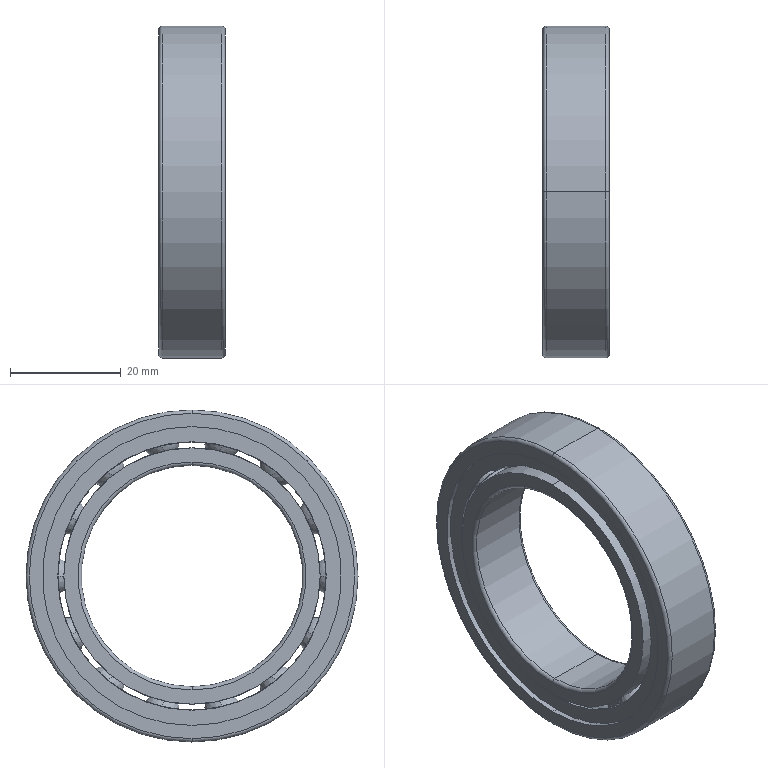Part | SolidWorks | 1 solid | 225 faces | box 12 x 60 x 60 mm | volume 12840 mm3 | sphere 112 | torus 53 | plane 36 | cylinder 24 | commonest cylinder face diameters 54 x8 46.3 x4 48.527 x4 40 x2 48.295 x2 52.005 x2